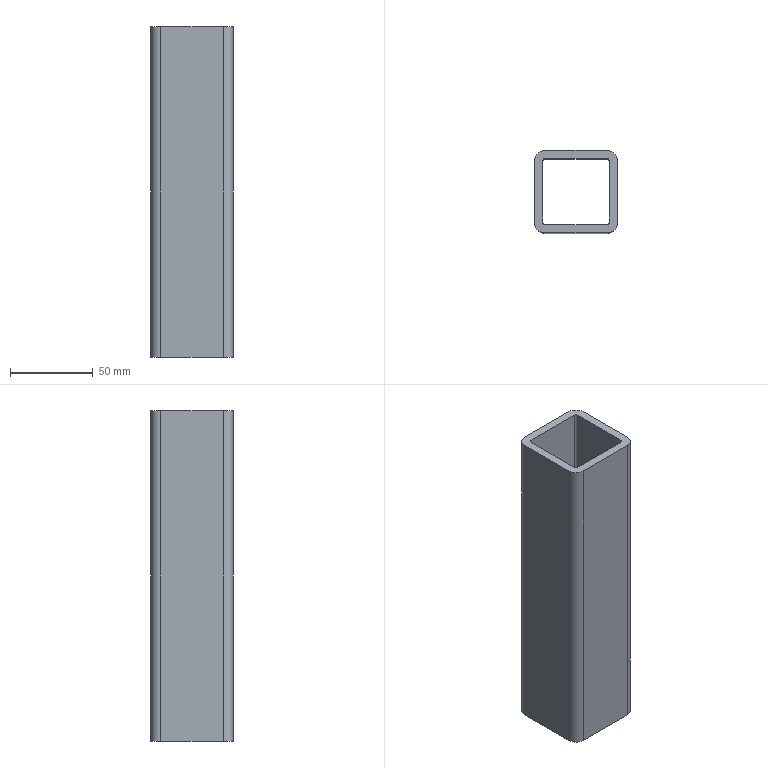Part | SolidWorks | features Extrusion 1 | 1 solid | 18 faces | box 50 x 50 x 200 mm | volume 173991 mm3 | plane 10 | cylinder 8 | commonest cylinder face diameters 2 x4 12 x4
STEP:
#1=CARTESIAN_POINT('',(0.,6.,200.));
#2=VERTEX_POINT('',#1);
#3=CARTESIAN_POINT('',(6.,0.,200.));
#4=VERTEX_POINT('',#3);
#5=CARTESIAN_POINT('',(6.,6.,200.));
#6=DIRECTION('',(0.,0.,1.));
#7=DIRECTION('',(-1.,0.,0.));
#8=AXIS2_PLACEMENT_3D('',#5,#6,#7);
#9=CIRCLE('',#8,6.);
#10=EDGE_CURVE('',#2,#4,#9,.T.);
#11=ORIENTED_EDGE('',*,*,#10,.T.);
#12=CARTESIAN_POINT('',(44.,0.,200.));
#13=VERTEX_POINT('',#12);
#14=CARTESIAN_POINT('',(6.,0.,200.));
#15=DIRECTION('',(1.,0.,0.));
#16=VECTOR('',#15,1000.);
#17=LINE('',#14,#16);
#18=EDGE_CURVE('',#4,#13,#17,.T.);
#19=ORIENTED_EDGE('',*,*,#18,.T.);
#20=CARTESIAN_POINT('',(50.,6.,200.));
#21=VERTEX_POINT('',#20);
#22=CARTESIAN_POINT('',(44.,6.,200.));
#23=DIRECTION('',(0.,0.,1.));
#24=DIRECTION('',(1.,0.,0.));
#25=AXIS2_PLACEMENT_3D('',#22,#23,#24);
#26=CIRCLE('',#25,6.);
#27=EDGE_CURVE('',#13,#21,#26,.T.);
#28=ORIENTED_EDGE('',*,*,#27,.T.);
#29=CARTESIAN_POINT('',(50.,44.,200.));
#30=VERTEX_POINT('',#29);
#31=CARTESIAN_POINT('',(50.,6.,200.));
#32=DIRECTION('',(0.,1.,0.));
#33=VECTOR('',#32,1000.);
#34=LINE('',#31,#33);
#35=EDGE_CURVE('',#21,#30,#34,.T.);
#36=ORIENTED_EDGE('',*,*,#35,.T.);
#37=CARTESIAN_POINT('',(44.,50.,200.));
#38=VERTEX_POINT('',#37);
#39=CARTESIAN_POINT('',(44.,44.,200.));
#40=DIRECTION('',(0.,0.,1.));
#41=DIRECTION('',(-1.,0.,0.));
#42=AXIS2_PLACEMENT_3D('',#39,#40,#41);
#43=CIRCLE('',#42,6.);
#44=EDGE_CURVE('',#30,#38,#43,.T.);
#45=ORIENTED_EDGE('',*,*,#44,.T.);
#46=CARTESIAN_POINT('',(6.,50.,200.));
#47=VERTEX_POINT('',#46);
#48=CARTESIAN_POINT('',(6.,50.,200.));
#49=DIRECTION('',(-1.,0.,0.));
#50=VECTOR('',#49,1000.);
#51=LINE('',#48,#50);
#52=EDGE_CURVE('',#38,#47,#51,.T.);
#53=ORIENTED_EDGE('',*,*,#52,.T.);
#54=CARTESIAN_POINT('',(0.,44.,200.));
#55=VERTEX_POINT('',#54);
#56=CARTESIAN_POINT('',(6.,44.,200.));
#57=DIRECTION('',(0.,0.,1.));
#58=DIRECTION('',(-1.,0.,0.));
#59=AXIS2_PLACEMENT_3D('',#56,#57,#58);
#60=CIRCLE('',#59,6.);
#61=EDGE_CURVE('',#47,#55,#60,.T.);
#62=ORIENTED_EDGE('',*,*,#61,.T.);
#63=CARTESIAN_POINT('',(0.,6.,200.));
#64=DIRECTION('',(0.,-1.,0.));
#65=VECTOR('',#64,1000.);
#66=LINE('',#63,#65);
#67=EDGE_CURVE('',#55,#2,#66,.T.);
#68=ORIENTED_EDGE('',*,*,#67,.T.);
#69=EDGE_LOOP('',(#11,#19,#28,#36,#45,#53,#62,#68));
#70=FACE_OUTER_BOUND('',#69,.T.);
#71=CARTESIAN_POINT('',(6.,45.,200.));
#72=VERTEX_POINT('',#71);
#73=CARTESIAN_POINT('',(5.,44.,200.));
#74=VERTEX_POINT('',#73);
#75=CARTESIAN_POINT('',(6.,44.,200.));
#76=DIRECTION('',(0.,0.,1.));
#77=DIRECTION('',(-1.,0.,0.));
#78=AXIS2_PLACEMENT_3D('',#75,#76,#77);
#79=CIRCLE('',#78,1.);
#80=EDGE_CURVE('',#72,#74,#79,.T.);
#81=ORIENTED_EDGE('',*,*,#80,.F.);
#82=CARTESIAN_POINT('',(44.,45.,200.));
#83=VERTEX_POINT('',#82);
#84=CARTESIAN_POINT('',(6.,45.,200.));
#85=DIRECTION('',(-1.,0.,0.));
#86=VECTOR('',#85,1000.);
#87=LINE('',#84,#86);
#88=EDGE_CURVE('',#83,#72,#87,.T.);
#89=ORIENTED_EDGE('',*,*,#88,.F.);
#90=CARTESIAN_POINT('',(45.,44.,200.));
#91=VERTEX_POINT('',#90);
#92=CARTESIAN_POINT('',(44.,44.,200.));
#93=DIRECTION('',(0.,0.,1.));
#94=DIRECTION('',(-1.,0.,0.));
#95=AXIS2_PLACEMENT_3D('',#92,#93,#94);
#96=CIRCLE('',#95,1.);
#97=EDGE_CURVE('',#91,#83,#96,.T.);
#98=ORIENTED_EDGE('',*,*,#97,.F.);
#99=CARTESIAN_POINT('',(45.,6.,200.));
#100=VERTEX_POINT('',#99);
#101=CARTESIAN_POINT('',(45.,6.,200.));
#102=DIRECTION('',(0.,1.,0.));
#103=VECTOR('',#102,1000.);
#104=LINE('',#101,#103);
#105=EDGE_CURVE('',#100,#91,#104,.T.);
#106=ORIENTED_EDGE('',*,*,#105,.F.);
#107=CARTESIAN_POINT('',(44.,5.,200.));
#108=VERTEX_POINT('',#107);
#109=CARTESIAN_POINT('',(44.,6.,200.));
#110=DIRECTION('',(0.,0.,1.));
#111=DIRECTION('',(1.,0.,0.));
#112=AXIS2_PLACEMENT_3D('',#109,#110,#111);
#113=CIRCLE('',#112,1.);
#114=EDGE_CURVE('',#108,#100,#113,.T.);
#115=ORIENTED_EDGE('',*,*,#114,.F.);
#116=CARTESIAN_POINT('',(6.,5.,200.));
#117=VERTEX_POINT('',#116);
#118=CARTESIAN_POINT('',(6.,5.,200.));
#119=DIRECTION('',(1.,0.,0.));
#120=VECTOR('',#119,1000.);
#121=LINE('',#118,#120);
#122=EDGE_CURVE('',#117,#108,#121,.T.);
#123=ORIENTED_EDGE('',*,*,#122,.F.);
#124=CARTESIAN_POINT('',(5.,6.,200.));
#125=VERTEX_POINT('',#124);
#126=CARTESIAN_POINT('',(6.,6.,200.));
#127=DIRECTION('',(0.,0.,1.));
#128=DIRECTION('',(-1.,0.,0.));
#129=AXIS2_PLACEMENT_3D('',#126,#127,#128);
#130=CIRCLE('',#129,1.);
#131=EDGE_CURVE('',#125,#117,#130,.T.);
#132=ORIENTED_EDGE('',*,*,#131,.F.);
#133=CARTESIAN_POINT('',(5.,6.,200.));
#134=DIRECTION('',(0.,-1.,0.));
#135=VECTOR('',#134,1000.);
#136=LINE('',#133,#135);
#137=EDGE_CURVE('',#74,#125,#136,.T.);
#138=ORIENTED_EDGE('',*,*,#137,.F.);
#139=EDGE_LOOP('',(#81,#89,#98,#106,#115,#123,#132,#138));
#140=FACE_BOUND('',#139,.T.);
#141=CARTESIAN_POINT('',(6.,6.,200.));
#142=DIRECTION('',(0.,0.,-1.));
#143=DIRECTION('',(-1.,0.,0.));
#144=AXIS2_PLACEMENT_3D('',#141,#142,#143);
#145=PLANE('',#144);
#146=ADVANCED_FACE('',(#70,#140),#145,.F.);
#147=CARTESIAN_POINT('',(0.,6.,0.));
#148=VERTEX_POINT('',#147);
#149=CARTESIAN_POINT('',(6.,0.,0.));
#150=VERTEX_POINT('',#149);
#151=CARTESIAN_POINT('',(6.,6.,0.));
#152=DIRECTION('',(0.,0.,1.));
#153=DIRECTION('',(-1.,0.,0.));
#154=AXIS2_PLACEMENT_3D('',#151,#152,#153);
#155=CIRCLE('',#154,6.);
#156=EDGE_CURVE('',#148,#150,#155,.T.);
#157=ORIENTED_EDGE('',*,*,#156,.F.);
#158=CARTESIAN_POINT('',(0.,44.,0.));
#159=VERTEX_POINT('',#158);
#160=CARTESIAN_POINT('',(0.,6.,0.));
#161=DIRECTION('',(0.,-1.,0.));
#162=VECTOR('',#161,1000.);
#163=LINE('',#160,#162);
#164=EDGE_CURVE('',#159,#148,#163,.T.);
#165=ORIENTED_EDGE('',*,*,#164,.F.);
#166=CARTESIAN_POINT('',(6.,50.,0.));
#167=VERTEX_POINT('',#166);
#168=CARTESIAN_POINT('',(6.,44.,0.));
#169=DIRECTION('',(0.,0.,1.));
#170=DIRECTION('',(-1.,0.,0.));
#171=AXIS2_PLACEMENT_3D('',#168,#169,#170);
#172=CIRCLE('',#171,6.);
#173=EDGE_CURVE('',#167,#159,#172,.T.);
#174=ORIENTED_EDGE('',*,*,#173,.F.);
#175=CARTESIAN_POINT('',(44.,50.,0.));
#176=VERTEX_POINT('',#175);
#177=CARTESIAN_POINT('',(6.,50.,0.));
#178=DIRECTION('',(-1.,0.,0.));
#179=VECTOR('',#178,1000.);
#180=LINE('',#177,#179);
#181=EDGE_CURVE('',#176,#167,#180,.T.);
#182=ORIENTED_EDGE('',*,*,#181,.F.);
#183=CARTESIAN_POINT('',(50.,44.,0.));
#184=VERTEX_POINT('',#183);
#185=CARTESIAN_POINT('',(44.,44.,0.));
#186=DIRECTION('',(0.,0.,1.));
#187=DIRECTION('',(-1.,0.,0.));
#188=AXIS2_PLACEMENT_3D('',#185,#186,#187);
#189=CIRCLE('',#188,6.);
#190=EDGE_CURVE('',#184,#176,#189,.T.);
#191=ORIENTED_EDGE('',*,*,#190,.F.);
#192=CARTESIAN_POINT('',(50.,6.,0.));
#193=VERTEX_POINT('',#192);
#194=CARTESIAN_POINT('',(50.,6.,0.));
#195=DIRECTION('',(0.,1.,0.));
#196=VECTOR('',#195,1000.);
#197=LINE('',#194,#196);
#198=EDGE_CURVE('',#193,#184,#197,.T.);
#199=ORIENTED_EDGE('',*,*,#198,.F.);
#200=CARTESIAN_POINT('',(44.,0.,0.));
#201=VERTEX_POINT('',#200);
#202=CARTESIAN_POINT('',(44.,6.,0.));
#203=DIRECTION('',(0.,0.,1.));
#204=DIRECTION('',(1.,0.,0.));
#205=AXIS2_PLACEMENT_3D('',#202,#203,#204);
#206=CIRCLE('',#205,6.);
#207=EDGE_CURVE('',#201,#193,#206,.T.);
#208=ORIENTED_EDGE('',*,*,#207,.F.);
#209=CARTESIAN_POINT('',(6.,0.,0.));
#210=DIRECTION('',(1.,0.,0.));
#211=VECTOR('',#210,1000.);
#212=LINE('',#209,#211);
#213=EDGE_CURVE('',#150,#201,#212,.T.);
#214=ORIENTED_EDGE('',*,*,#213,.F.);
#215=EDGE_LOOP('',(#157,#165,#174,#182,#191,#199,#208,#214));
#216=FACE_OUTER_BOUND('',#215,.T.);
#217=CARTESIAN_POINT('',(44.,45.,0.));
#218=VERTEX_POINT('',#217);
#219=CARTESIAN_POINT('',(6.,45.,0.));
#220=VERTEX_POINT('',#219);
#221=CARTESIAN_POINT('',(6.,45.,0.));
#222=DIRECTION('',(-1.,0.,0.));
#223=VECTOR('',#222,1000.);
#224=LINE('',#221,#223);
#225=EDGE_CURVE('',#218,#220,#224,.T.);
#226=ORIENTED_EDGE('',*,*,#225,.T.);
#227=CARTESIAN_POINT('',(5.,44.,0.));
#228=VERTEX_POINT('',#227);
#229=CARTESIAN_POINT('',(6.,44.,0.));
#230=DIRECTION('',(0.,0.,1.));
#231=DIRECTION('',(-1.,0.,0.));
#232=AXIS2_PLACEMENT_3D('',#229,#230,#231);
#233=CIRCLE('',#232,1.);
#234=EDGE_CURVE('',#220,#228,#233,.T.);
#235=ORIENTED_EDGE('',*,*,#234,.T.);
#236=CARTESIAN_POINT('',(5.,6.,0.));
#237=VERTEX_POINT('',#236);
#238=CARTESIAN_POINT('',(5.,6.,0.));
#239=DIRECTION('',(0.,-1.,0.));
#240=VECTOR('',#239,1000.);
#241=LINE('',#238,#240);
#242=EDGE_CURVE('',#228,#237,#241,.T.);
#243=ORIENTED_EDGE('',*,*,#242,.T.);
#244=CARTESIAN_POINT('',(6.,5.,0.));
#245=VERTEX_POINT('',#244);
#246=CARTESIAN_POINT('',(6.,6.,0.));
#247=DIRECTION('',(0.,0.,1.));
#248=DIRECTION('',(-1.,0.,0.));
#249=AXIS2_PLACEMENT_3D('',#246,#247,#248);
#250=CIRCLE('',#249,1.);
#251=EDGE_CURVE('',#237,#245,#250,.T.);
#252=ORIENTED_EDGE('',*,*,#251,.T.);
#253=CARTESIAN_POINT('',(44.,5.,0.));
#254=VERTEX_POINT('',#253);
#255=CARTESIAN_POINT('',(6.,5.,0.));
#256=DIRECTION('',(1.,0.,0.));
#257=VECTOR('',#256,1000.);
#258=LINE('',#255,#257);
#259=EDGE_CURVE('',#245,#254,#258,.T.);
#260=ORIENTED_EDGE('',*,*,#259,.T.);
#261=CARTESIAN_POINT('',(45.,6.,0.));
#262=VERTEX_POINT('',#261);
#263=CARTESIAN_POINT('',(44.,6.,0.));
#264=DIRECTION('',(0.,0.,1.));
#265=DIRECTION('',(1.,0.,0.));
#266=AXIS2_PLACEMENT_3D('',#263,#264,#265);
#267=CIRCLE('',#266,1.);
#268=EDGE_CURVE('',#254,#262,#267,.T.);
#269=ORIENTED_EDGE('',*,*,#268,.T.);
#270=CARTESIAN_POINT('',(45.,44.,0.));
#271=VERTEX_POINT('',#270);
#272=CARTESIAN_POINT('',(45.,6.,0.));
#273=DIRECTION('',(0.,1.,0.));
#274=VECTOR('',#273,1000.);
#275=LINE('',#272,#274);
#276=EDGE_CURVE('',#262,#271,#275,.T.);
#277=ORIENTED_EDGE('',*,*,#276,.T.);
#278=CARTESIAN_POINT('',(44.,44.,0.));
#279=DIRECTION('',(0.,0.,1.));
#280=DIRECTION('',(-1.,0.,0.));
#281=AXIS2_PLACEMENT_3D('',#278,#279,#280);
#282=CIRCLE('',#281,1.);
#283=EDGE_CURVE('',#271,#218,#282,.T.);
#284=ORIENTED_EDGE('',*,*,#283,.T.);
#285=EDGE_LOOP('',(#226,#235,#243,#252,#260,#269,#277,#284));
#286=FACE_BOUND('',#285,.T.);
#287=CARTESIAN_POINT('',(6.,6.,0.));
#288=DIRECTION('',(0.,0.,-1.));
#289=DIRECTION('',(-1.,0.,0.));
#290=AXIS2_PLACEMENT_3D('',#287,#288,#289);
#291=PLANE('',#290);
#292=ADVANCED_FACE('',(#216,#286),#291,.T.);
#293=ORIENTED_EDGE('',*,*,#156,.T.);
#294=CARTESIAN_POINT('',(6.,0.,200.));
#295=DIRECTION('',(0.,0.,-1.));
#296=VECTOR('',#295,1000.);
#297=LINE('',#294,#296);
#298=EDGE_CURVE('',#4,#150,#297,.T.);
#299=ORIENTED_EDGE('',*,*,#298,.F.);
#300=ORIENTED_EDGE('',*,*,#10,.F.);
#301=CARTESIAN_POINT('',(0.,6.,200.));
#302=DIRECTION('',(0.,0.,-1.));
#303=VECTOR('',#302,1000.);
#304=LINE('',#301,#303);
#305=EDGE_CURVE('',#2,#148,#304,.T.);
#306=ORIENTED_EDGE('',*,*,#305,.T.);
#307=EDGE_LOOP('',(#293,#299,#300,#306));
#308=FACE_OUTER_BOUND('',#307,.T.);
#309=CARTESIAN_POINT('',(6.,6.,200.));
#310=DIRECTION('',(0.,0.,-1.));
#311=DIRECTION('',(-1.,0.,0.));
#312=AXIS2_PLACEMENT_3D('',#309,#310,#311);
#313=CYLINDRICAL_SURFACE('',#312,6.);
#314=ADVANCED_FACE('',(#308),#313,.T.);
#315=ORIENTED_EDGE('',*,*,#213,.T.);
#316=CARTESIAN_POINT('',(44.,0.,200.));
#317=DIRECTION('',(0.,0.,-1.));
#318=VECTOR('',#317,1000.);
#319=LINE('',#316,#318);
#320=EDGE_CURVE('',#13,#201,#319,.T.);
#321=ORIENTED_EDGE('',*,*,#320,.F.);
#322=ORIENTED_EDGE('',*,*,#18,.F.);
#323=ORIENTED_EDGE('',*,*,#298,.T.);
#324=EDGE_LOOP('',(#315,#321,#322,#323));
#325=FACE_OUTER_BOUND('',#324,.T.);
#326=CARTESIAN_POINT('',(6.,0.,200.));
#327=DIRECTION('',(0.,1.,0.));
#328=DIRECTION('',(0.,0.,1.));
#329=AXIS2_PLACEMENT_3D('',#326,#327,#328);
#330=PLANE('',#329);
#331=ADVANCED_FACE('',(#325),#330,.F.);
#332=ORIENTED_EDGE('',*,*,#207,.T.);
#333=CARTESIAN_POINT('',(50.,6.,200.));
#334=DIRECTION('',(0.,0.,-1.));
#335=VECTOR('',#334,1000.);
#336=LINE('',#333,#335);
#337=EDGE_CURVE('',#21,#193,#336,.T.);
#338=ORIENTED_EDGE('',*,*,#337,.F.);
#339=ORIENTED_EDGE('',*,*,#27,.F.);
#340=ORIENTED_EDGE('',*,*,#320,.T.);
#341=EDGE_LOOP('',(#332,#338,#339,#340));
#342=FACE_OUTER_BOUND('',#341,.T.);
#343=CARTESIAN_POINT('',(44.,6.,200.));
#344=DIRECTION('',(0.,0.,-1.));
#345=DIRECTION('',(-1.,0.,0.));
#346=AXIS2_PLACEMENT_3D('',#343,#344,#345);
#347=CYLINDRICAL_SURFACE('',#346,6.);
#348=ADVANCED_FACE('',(#342),#347,.T.);
#349=ORIENTED_EDGE('',*,*,#198,.T.);
#350=CARTESIAN_POINT('',(50.,44.,200.));
#351=DIRECTION('',(0.,0.,-1.));
#352=VECTOR('',#351,1000.);
#353=LINE('',#350,#352);
#354=EDGE_CURVE('',#30,#184,#353,.T.);
#355=ORIENTED_EDGE('',*,*,#354,.F.);
#356=ORIENTED_EDGE('',*,*,#35,.F.);
#357=ORIENTED_EDGE('',*,*,#337,.T.);
#358=EDGE_LOOP('',(#349,#355,#356,#357));
#359=FACE_OUTER_BOUND('',#358,.T.);
#360=CARTESIAN_POINT('',(50.,6.,200.));
#361=DIRECTION('',(-1.,0.,0.));
#362=DIRECTION('',(0.,0.,1.));
#363=AXIS2_PLACEMENT_3D('',#360,#361,#362);
#364=PLANE('',#363);
#365=ADVANCED_FACE('',(#359),#364,.F.);
#366=ORIENTED_EDGE('',*,*,#190,.T.);
#367=CARTESIAN_POINT('',(44.,50.,200.));
#368=DIRECTION('',(0.,0.,-1.));
#369=VECTOR('',#368,1000.);
#370=LINE('',#367,#369);
#371=EDGE_CURVE('',#38,#176,#370,.T.);
#372=ORIENTED_EDGE('',*,*,#371,.F.);
#373=ORIENTED_EDGE('',*,*,#44,.F.);
#374=ORIENTED_EDGE('',*,*,#354,.T.);
#375=EDGE_LOOP('',(#366,#372,#373,#374));
#376=FACE_OUTER_BOUND('',#375,.T.);
#377=CARTESIAN_POINT('',(44.,44.,200.));
#378=DIRECTION('',(0.,0.,-1.));
#379=DIRECTION('',(-1.,0.,0.));
#380=AXIS2_PLACEMENT_3D('',#377,#378,#379);
#381=CYLINDRICAL_SURFACE('',#380,6.);
#382=ADVANCED_FACE('',(#376),#381,.T.);
#383=ORIENTED_EDGE('',*,*,#181,.T.);
#384=CARTESIAN_POINT('',(6.,50.,200.));
#385=DIRECTION('',(0.,0.,-1.));
#386=VECTOR('',#385,1000.);
#387=LINE('',#384,#386);
#388=EDGE_CURVE('',#47,#167,#387,.T.);
#389=ORIENTED_EDGE('',*,*,#388,.F.);
#390=ORIENTED_EDGE('',*,*,#52,.F.);
#391=ORIENTED_EDGE('',*,*,#371,.T.);
#392=EDGE_LOOP('',(#383,#389,#390,#391));
#393=FACE_OUTER_BOUND('',#392,.T.);
#394=CARTESIAN_POINT('',(6.,50.,200.));
#395=DIRECTION('',(0.,-1.,0.));
#396=DIRECTION('',(0.,0.,-1.));
#397=AXIS2_PLACEMENT_3D('',#394,#395,#396);
#398=PLANE('',#397);
#399=ADVANCED_FACE('',(#393),#398,.F.);
#400=ORIENTED_EDGE('',*,*,#173,.T.);
#401=CARTESIAN_POINT('',(0.,44.,200.));
#402=DIRECTION('',(0.,0.,-1.));
#403=VECTOR('',#402,1000.);
#404=LINE('',#401,#403);
#405=EDGE_CURVE('',#55,#159,#404,.T.);
#406=ORIENTED_EDGE('',*,*,#405,.F.);
#407=ORIENTED_EDGE('',*,*,#61,.F.);
#408=ORIENTED_EDGE('',*,*,#388,.T.);
#409=EDGE_LOOP('',(#400,#406,#407,#408));
#410=FACE_OUTER_BOUND('',#409,.T.);
#411=CARTESIAN_POINT('',(6.,44.,200.));
#412=DIRECTION('',(0.,0.,-1.));
#413=DIRECTION('',(-1.,0.,0.));
#414=AXIS2_PLACEMENT_3D('',#411,#412,#413);
#415=CYLINDRICAL_SURFACE('',#414,6.);
#416=ADVANCED_FACE('',(#410),#415,.T.);
#417=ORIENTED_EDGE('',*,*,#164,.T.);
#418=ORIENTED_EDGE('',*,*,#305,.F.);
#419=ORIENTED_EDGE('',*,*,#67,.F.);
#420=ORIENTED_EDGE('',*,*,#405,.T.);
#421=EDGE_LOOP('',(#417,#418,#419,#420));
#422=FACE_OUTER_BOUND('',#421,.T.);
#423=CARTESIAN_POINT('',(0.,6.,200.));
#424=DIRECTION('',(1.,0.,0.));
#425=DIRECTION('',(0.,0.,-1.));
#426=AXIS2_PLACEMENT_3D('',#423,#424,#425);
#427=PLANE('',#426);
#428=ADVANCED_FACE('',(#422),#427,.F.);
#429=ORIENTED_EDGE('',*,*,#234,.F.);
#430=CARTESIAN_POINT('',(6.,45.,200.));
#431=DIRECTION('',(0.,0.,-1.));
#432=VECTOR('',#431,1000.);
#433=LINE('',#430,#432);
#434=EDGE_CURVE('',#72,#220,#433,.T.);
#435=ORIENTED_EDGE('',*,*,#434,.F.);
#436=ORIENTED_EDGE('',*,*,#80,.T.);
#437=CARTESIAN_POINT('',(5.,44.,200.));
#438=DIRECTION('',(0.,0.,-1.));
#439=VECTOR('',#438,1000.);
#440=LINE('',#437,#439);
#441=EDGE_CURVE('',#74,#228,#440,.T.);
#442=ORIENTED_EDGE('',*,*,#441,.T.);
#443=EDGE_LOOP('',(#429,#435,#436,#442));
#444=FACE_OUTER_BOUND('',#443,.T.);
#445=CARTESIAN_POINT('',(6.,44.,200.));
#446=DIRECTION('',(0.,0.,-1.));
#447=DIRECTION('',(-1.,0.,0.));
#448=AXIS2_PLACEMENT_3D('',#445,#446,#447);
#449=CYLINDRICAL_SURFACE('',#448,1.);
#450=ADVANCED_FACE('',(#444),#449,.F.);
#451=ORIENTED_EDGE('',*,*,#242,.F.);
#452=ORIENTED_EDGE('',*,*,#441,.F.);
#453=ORIENTED_EDGE('',*,*,#137,.T.);
#454=CARTESIAN_POINT('',(5.,6.,200.));
#455=DIRECTION('',(0.,0.,-1.));
#456=VECTOR('',#455,1000.);
#457=LINE('',#454,#456);
#458=EDGE_CURVE('',#125,#237,#457,.T.);
#459=ORIENTED_EDGE('',*,*,#458,.T.);
#460=EDGE_LOOP('',(#451,#452,#453,#459));
#461=FACE_OUTER_BOUND('',#460,.T.);
#462=CARTESIAN_POINT('',(5.,6.,200.));
#463=DIRECTION('',(1.,0.,0.));
#464=DIRECTION('',(0.,1.,0.));
#465=AXIS2_PLACEMENT_3D('',#462,#463,#464);
#466=PLANE('',#465);
#467=ADVANCED_FACE('',(#461),#466,.T.);
#468=ORIENTED_EDGE('',*,*,#251,.F.);
#469=ORIENTED_EDGE('',*,*,#458,.F.);
#470=ORIENTED_EDGE('',*,*,#131,.T.);
#471=CARTESIAN_POINT('',(6.,5.,200.));
#472=DIRECTION('',(0.,0.,-1.));
#473=VECTOR('',#472,1000.);
#474=LINE('',#471,#473);
#475=EDGE_CURVE('',#117,#245,#474,.T.);
#476=ORIENTED_EDGE('',*,*,#475,.T.);
#477=EDGE_LOOP('',(#468,#469,#470,#476));
#478=FACE_OUTER_BOUND('',#477,.T.);
#479=CARTESIAN_POINT('',(6.,6.,200.));
#480=DIRECTION('',(0.,0.,-1.));
#481=DIRECTION('',(-1.,0.,0.));
#482=AXIS2_PLACEMENT_3D('',#479,#480,#481);
#483=CYLINDRICAL_SURFACE('',#482,1.);
#484=ADVANCED_FACE('',(#478),#483,.F.);
#485=ORIENTED_EDGE('',*,*,#259,.F.);
#486=ORIENTED_EDGE('',*,*,#475,.F.);
#487=ORIENTED_EDGE('',*,*,#122,.T.);
#488=CARTESIAN_POINT('',(44.,5.,200.));
#489=DIRECTION('',(0.,0.,-1.));
#490=VECTOR('',#489,1000.);
#491=LINE('',#488,#490);
#492=EDGE_CURVE('',#108,#254,#491,.T.);
#493=ORIENTED_EDGE('',*,*,#492,.T.);
#494=EDGE_LOOP('',(#485,#486,#487,#493));
#495=FACE_OUTER_BOUND('',#494,.T.);
#496=CARTESIAN_POINT('',(6.,5.,200.));
#497=DIRECTION('',(0.,1.,0.));
#498=DIRECTION('',(-1.,0.,0.));
#499=AXIS2_PLACEMENT_3D('',#496,#497,#498);
#500=PLANE('',#499);
#501=ADVANCED_FACE('',(#495),#500,.T.);
#502=ORIENTED_EDGE('',*,*,#268,.F.);
#503=ORIENTED_EDGE('',*,*,#492,.F.);
#504=ORIENTED_EDGE('',*,*,#114,.T.);
#505=CARTESIAN_POINT('',(45.,6.,200.));
#506=DIRECTION('',(0.,0.,-1.));
#507=VECTOR('',#506,1000.);
#508=LINE('',#505,#507);
#509=EDGE_CURVE('',#100,#262,#508,.T.);
#510=ORIENTED_EDGE('',*,*,#509,.T.);
#511=EDGE_LOOP('',(#502,#503,#504,#510));
#512=FACE_OUTER_BOUND('',#511,.T.);
#513=CARTESIAN_POINT('',(44.,6.,200.));
#514=DIRECTION('',(0.,0.,-1.));
#515=DIRECTION('',(-1.,0.,0.));
#516=AXIS2_PLACEMENT_3D('',#513,#514,#515);
#517=CYLINDRICAL_SURFACE('',#516,1.);
#518=ADVANCED_FACE('',(#512),#517,.F.);
#519=ORIENTED_EDGE('',*,*,#276,.F.);
#520=ORIENTED_EDGE('',*,*,#509,.F.);
#521=ORIENTED_EDGE('',*,*,#105,.T.);
#522=CARTESIAN_POINT('',(45.,44.,200.));
#523=DIRECTION('',(0.,0.,-1.));
#524=VECTOR('',#523,1000.);
#525=LINE('',#522,#524);
#526=EDGE_CURVE('',#91,#271,#525,.T.);
#527=ORIENTED_EDGE('',*,*,#526,.T.);
#528=EDGE_LOOP('',(#519,#520,#521,#527));
#529=FACE_OUTER_BOUND('',#528,.T.);
#530=CARTESIAN_POINT('',(45.,6.,200.));
#531=DIRECTION('',(-1.,0.,0.));
#532=DIRECTION('',(0.,0.,1.));
#533=AXIS2_PLACEMENT_3D('',#530,#531,#532);
#534=PLANE('',#533);
#535=ADVANCED_FACE('',(#529),#534,.T.);
#536=ORIENTED_EDGE('',*,*,#283,.F.);
#537=ORIENTED_EDGE('',*,*,#526,.F.);
#538=ORIENTED_EDGE('',*,*,#97,.T.);
#539=CARTESIAN_POINT('',(44.,45.,200.));
#540=DIRECTION('',(0.,0.,-1.));
#541=VECTOR('',#540,1000.);
#542=LINE('',#539,#541);
#543=EDGE_CURVE('',#83,#218,#542,.T.);
#544=ORIENTED_EDGE('',*,*,#543,.T.);
#545=EDGE_LOOP('',(#536,#537,#538,#544));
#546=FACE_OUTER_BOUND('',#545,.T.);
#547=CARTESIAN_POINT('',(44.,44.,200.));
#548=DIRECTION('',(0.,0.,-1.));
#549=DIRECTION('',(-1.,0.,0.));
#550=AXIS2_PLACEMENT_3D('',#547,#548,#549);
#551=CYLINDRICAL_SURFACE('',#550,1.);
#552=ADVANCED_FACE('',(#546),#551,.F.);
#553=ORIENTED_EDGE('',*,*,#225,.F.);
#554=ORIENTED_EDGE('',*,*,#543,.F.);
#555=ORIENTED_EDGE('',*,*,#88,.T.);
#556=ORIENTED_EDGE('',*,*,#434,.T.);
#557=EDGE_LOOP('',(#553,#554,#555,#556));
#558=FACE_OUTER_BOUND('',#557,.T.);
#559=CARTESIAN_POINT('',(6.,45.,200.));
#560=DIRECTION('',(0.,-1.,0.));
#561=DIRECTION('',(0.,0.,-1.));
#562=AXIS2_PLACEMENT_3D('',#559,#560,#561);
#563=PLANE('',#562);
#564=ADVANCED_FACE('',(#558),#563,.T.);
#565=CLOSED_SHELL('',(#146,#292,#314,#331,#348,#365,#382,#399,#416,#428,#450,#467,#484,#501,#518,#535,#552,#564));
#566=MANIFOLD_SOLID_BREP('',#565);
#567=CARTESIAN_POINT('',(0.,0.,0.));
#568=DIRECTION('',(0.,0.,1.));
#569=DIRECTION('',(1.,0.,0.));
#570=AXIS2_PLACEMENT_3D('',#567,#568,#569);
#571=(LENGTH_UNIT()NAMED_UNIT(*)SI_UNIT(.MILLI.,.METRE.));
#572=UNCERTAINTY_MEASURE_WITH_UNIT(LENGTH_MEASURE(0.00001),#571,'','');
#573=(NAMED_UNIT(*)PLANE_ANGLE_UNIT()SI_UNIT($,.RADIAN.));
#574=(NAMED_UNIT(*)SI_UNIT($,.STERADIAN.)SOLID_ANGLE_UNIT());
#575=(GEOMETRIC_REPRESENTATION_CONTEXT(3)GLOBAL_UNCERTAINTY_ASSIGNED_CONTEXT((#572))GLOBAL_UNIT_ASSIGNED_CONTEXT((#571,#573,#574))REPRESENTATION_CONTEXT('',''));
#576=ADVANCED_BREP_SHAPE_REPRESENTATION('',(#566,#570),#575);